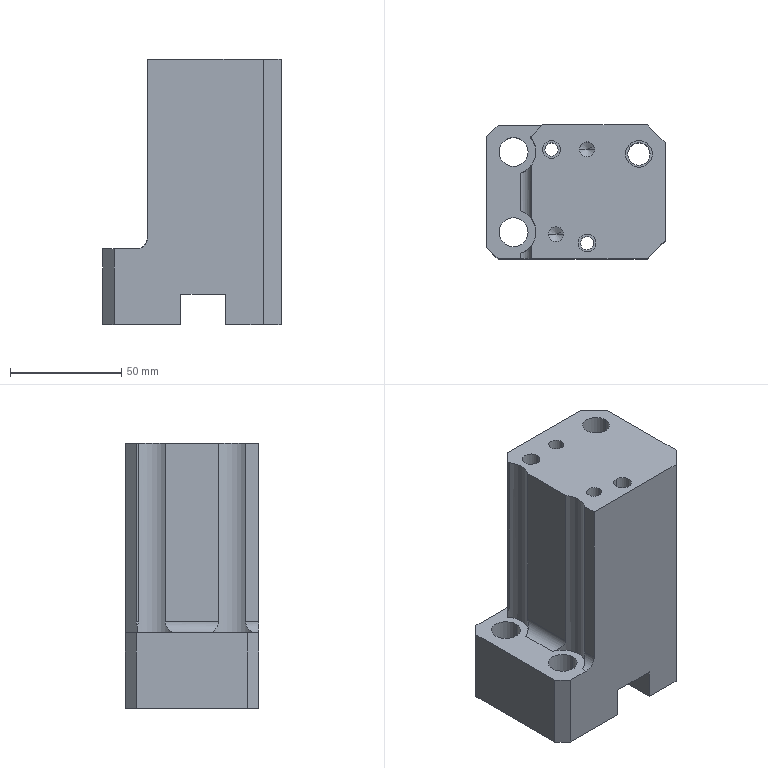Part | STEP file | 1_id818_x_t | 1 solid | 57 faces | box 80 x 60 x 119 mm | volume 412634 mm3 | cylinder 27 | plane 22 | cone 8 | commonest cylinder face diameters 10 x5 6 x4 6.75 x4 8 x4 13 x4 6.528 x2